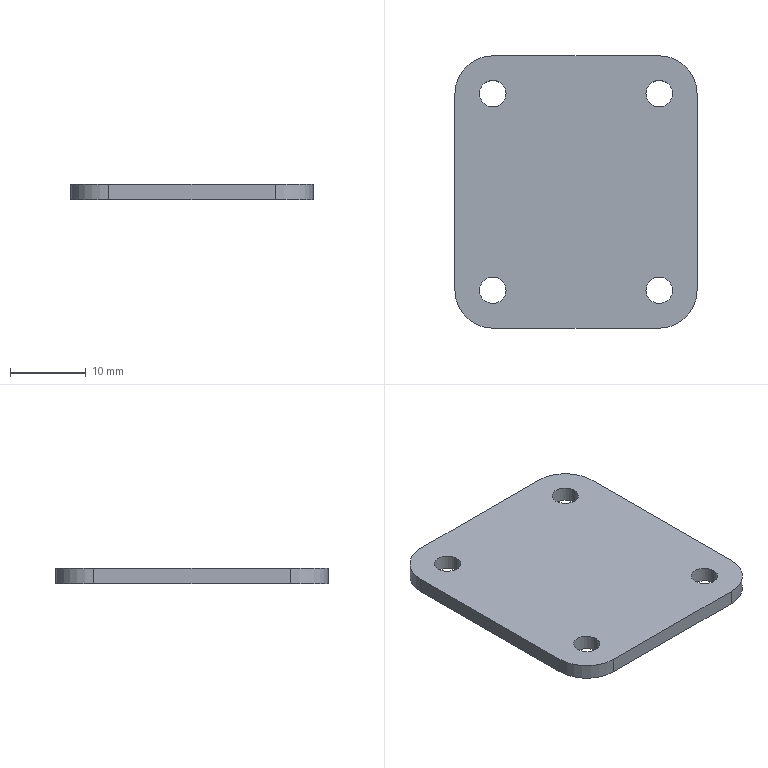Part | STEP file | YCD14007A-08.03.08.05 Engraving Plate | 1 solid | 18 faces | box 32 x 36 x 2 mm | volume 2184 mm3 | cylinder 12 | plane 6 | commonest cylinder face diameters 3.5 x8 10 x4
STEP:
#1=CARTESIAN_POINT('',(0.,0.,0.));
#2=DIRECTION('',(0.,0.,1.));
#3=DIRECTION('',(1.,0.,0.));
#4=AXIS2_PLACEMENT_3D('',#1,#2,#3);
#5=CARTESIAN_POINT('',(12.75,-13.,0.));
#6=VERTEX_POINT('',#5);
#7=CARTESIAN_POINT('',(12.75,-13.,2.));
#8=VERTEX_POINT('',#7);
#9=CARTESIAN_POINT('',(12.75,-13.,-0.001));
#10=DIRECTION('',(0.,0.,1.));
#11=VECTOR('',#10,1.);
#12=LINE('',#9,#11);
#13=CARTESIAN_POINT('',(11.,-13.,-0.001));
#14=DIRECTION('',(0.,0.,1.));
#15=DIRECTION('',(1.,0.,0.));
#16=AXIS2_PLACEMENT_3D('',#13,#14,#15);
#17=CYLINDRICAL_SURFACE('',#16,1.75);
#18=CARTESIAN_POINT('',(6.283,0.));
#19=DIRECTION('',(0.,1.));
#20=VECTOR('',#19,1.);
#21=LINE('',#18,#20);
#22=(GEOMETRIC_REPRESENTATION_CONTEXT(2)PARAMETRIC_REPRESENTATION_CONTEXT()REPRESENTATION_CONTEXT('',''));
#23=DEFINITIONAL_REPRESENTATION('',(#21),#22);
#24=PCURVE('',#17,#23);
#25=CARTESIAN_POINT('',(11.,-13.,-0.001));
#26=DIRECTION('',(0.,0.,1.));
#27=DIRECTION('',(1.,0.,0.));
#28=AXIS2_PLACEMENT_3D('',#25,#26,#27);
#29=CYLINDRICAL_SURFACE('',#28,1.75);
#30=CARTESIAN_POINT('',(0.,0.));
#31=DIRECTION('',(0.,1.));
#32=VECTOR('',#31,1.);
#33=LINE('',#30,#32);
#34=(GEOMETRIC_REPRESENTATION_CONTEXT(2)PARAMETRIC_REPRESENTATION_CONTEXT()REPRESENTATION_CONTEXT('',''));
#35=DEFINITIONAL_REPRESENTATION('',(#33),#34);
#36=PCURVE('',#29,#35);
#37=SURFACE_CURVE('',#12,(#24,#36),.PCURVE_S1.);
#38=EDGE_CURVE('',#6,#8,#37,.T.);
#39=ORIENTED_EDGE('',*,*,#38,.T.);
#40=CARTESIAN_POINT('',(9.25,-13.,2.));
#41=VERTEX_POINT('',#40);
#42=CARTESIAN_POINT('',(11.,-13.,2.));
#43=DIRECTION('',(0.,0.,1.));
#44=DIRECTION('',(1.,0.,0.));
#45=AXIS2_PLACEMENT_3D('',#42,#43,#44);
#46=CIRCLE('',#45,1.75);
#47=CARTESIAN_POINT('',(0.,2.001));
#48=DIRECTION('',(1.,0.));
#49=VECTOR('',#48,1.);
#50=LINE('',#47,#49);
#51=(GEOMETRIC_REPRESENTATION_CONTEXT(2)PARAMETRIC_REPRESENTATION_CONTEXT()REPRESENTATION_CONTEXT('',''));
#52=DEFINITIONAL_REPRESENTATION('',(#50),#51);
#53=PCURVE('',#17,#52);
#54=CARTESIAN_POINT('',(0.,0.,2.));
#55=DIRECTION('',(0.,0.,1.));
#56=DIRECTION('',(1.,0.,0.));
#57=AXIS2_PLACEMENT_3D('',#54,#55,#56);
#58=PLANE('',#57);
#59=CARTESIAN_POINT('',(11.,-13.));
#60=DIRECTION('',(1.,0.));
#61=AXIS2_PLACEMENT_2D('',#59,#60);
#62=CIRCLE('',#61,1.75);
#63=(GEOMETRIC_REPRESENTATION_CONTEXT(2)PARAMETRIC_REPRESENTATION_CONTEXT()REPRESENTATION_CONTEXT('',''));
#64=DEFINITIONAL_REPRESENTATION('',(#62),#63);
#65=PCURVE('',#58,#64);
#66=SURFACE_CURVE('',#46,(#53,#65),.PCURVE_S1.);
#67=EDGE_CURVE('',#41,#8,#66,.T.);
#68=ORIENTED_EDGE('',*,*,#67,.F.);
#69=CARTESIAN_POINT('',(9.25,-13.,0.));
#70=VERTEX_POINT('',#69);
#71=CARTESIAN_POINT('',(9.25,-13.,-0.001));
#72=DIRECTION('',(0.,0.,1.));
#73=VECTOR('',#72,1.);
#74=LINE('',#71,#73);
#75=CARTESIAN_POINT('',(3.142,0.));
#76=DIRECTION('',(0.,1.));
#77=VECTOR('',#76,1.);
#78=LINE('',#75,#77);
#79=(GEOMETRIC_REPRESENTATION_CONTEXT(2)PARAMETRIC_REPRESENTATION_CONTEXT()REPRESENTATION_CONTEXT('',''));
#80=DEFINITIONAL_REPRESENTATION('',(#78),#79);
#81=PCURVE('',#17,#80);
#82=CARTESIAN_POINT('',(3.142,0.));
#83=DIRECTION('',(0.,1.));
#84=VECTOR('',#83,1.);
#85=LINE('',#82,#84);
#86=(GEOMETRIC_REPRESENTATION_CONTEXT(2)PARAMETRIC_REPRESENTATION_CONTEXT()REPRESENTATION_CONTEXT('',''));
#87=DEFINITIONAL_REPRESENTATION('',(#85),#86);
#88=PCURVE('',#29,#87);
#89=SURFACE_CURVE('',#74,(#81,#88),.PCURVE_S1.);
#90=EDGE_CURVE('',#70,#41,#89,.T.);
#91=ORIENTED_EDGE('',*,*,#90,.F.);
#92=CARTESIAN_POINT('',(11.,-13.,0.));
#93=DIRECTION('',(0.,0.,-1.));
#94=DIRECTION('',(1.,0.,0.));
#95=AXIS2_PLACEMENT_3D('',#92,#93,#94);
#96=CIRCLE('',#95,1.75);
#97=CARTESIAN_POINT('',(6.283,0.001));
#98=DIRECTION('',(-1.,0.));
#99=VECTOR('',#98,1.);
#100=LINE('',#97,#99);
#101=(GEOMETRIC_REPRESENTATION_CONTEXT(2)PARAMETRIC_REPRESENTATION_CONTEXT()REPRESENTATION_CONTEXT('',''));
#102=DEFINITIONAL_REPRESENTATION('',(#100),#101);
#103=PCURVE('',#17,#102);
#104=CARTESIAN_POINT('',(0.,0.,0.));
#105=DIRECTION('',(0.,0.,1.));
#106=DIRECTION('',(1.,0.,0.));
#107=AXIS2_PLACEMENT_3D('',#104,#105,#106);
#108=PLANE('',#107);
#109=CARTESIAN_POINT('',(12.75,-13.));
#110=CARTESIAN_POINT('',(12.75,-16.031));
#111=CARTESIAN_POINT('',(10.125,-14.516));
#112=CARTESIAN_POINT('',(7.5,-13.));
#113=CARTESIAN_POINT('',(10.125,-11.484));
#114=CARTESIAN_POINT('',(12.75,-9.969));
#115=CARTESIAN_POINT('',(12.75,-13.));
#116=(BOUNDED_CURVE()B_SPLINE_CURVE(2,(#109,#110,#111,#112,#113,#114,#115),.UNSPECIFIED.,.T.,.F.)B_SPLINE_CURVE_WITH_KNOTS((1,2,2,2,2,1),(-2.094,0.,2.094,4.189,6.283,8.378),.UNSPECIFIED.)CURVE()GEOMETRIC_REPRESENTATION_ITEM()RATIONAL_B_SPLINE_CURVE((1.,0.5,1.,0.5,1.,0.5,1.))REPRESENTATION_ITEM(''));
#117=(GEOMETRIC_REPRESENTATION_CONTEXT(2)PARAMETRIC_REPRESENTATION_CONTEXT()REPRESENTATION_CONTEXT('',''));
#118=DEFINITIONAL_REPRESENTATION('',(#116),#117);
#119=PCURVE('',#108,#118);
#120=SURFACE_CURVE('',#96,(#103,#119),.PCURVE_S1.);
#121=EDGE_CURVE('',#6,#70,#120,.T.);
#122=ORIENTED_EDGE('',*,*,#121,.F.);
#123=EDGE_LOOP('',(#39,#68,#91,#122));
#124=FACE_BOUND('',#123,.F.);
#125=ADVANCED_FACE('',(#124),#17,.F.);
#126=CARTESIAN_POINT('',(-9.25,-13.,0.));
#127=VERTEX_POINT('',#126);
#128=CARTESIAN_POINT('',(-9.25,-13.,2.));
#129=VERTEX_POINT('',#128);
#130=CARTESIAN_POINT('',(-9.25,-13.,-0.001));
#131=DIRECTION('',(0.,0.,1.));
#132=VECTOR('',#131,1.);
#133=LINE('',#130,#132);
#134=CARTESIAN_POINT('',(-11.,-13.,-0.001));
#135=DIRECTION('',(0.,0.,1.));
#136=DIRECTION('',(1.,0.,0.));
#137=AXIS2_PLACEMENT_3D('',#134,#135,#136);
#138=CYLINDRICAL_SURFACE('',#137,1.75);
#139=CARTESIAN_POINT('',(6.283,0.));
#140=DIRECTION('',(0.,1.));
#141=VECTOR('',#140,1.);
#142=LINE('',#139,#141);
#143=(GEOMETRIC_REPRESENTATION_CONTEXT(2)PARAMETRIC_REPRESENTATION_CONTEXT()REPRESENTATION_CONTEXT('',''));
#144=DEFINITIONAL_REPRESENTATION('',(#142),#143);
#145=PCURVE('',#138,#144);
#146=CARTESIAN_POINT('',(-11.,-13.,-0.001));
#147=DIRECTION('',(0.,0.,1.));
#148=DIRECTION('',(1.,0.,0.));
#149=AXIS2_PLACEMENT_3D('',#146,#147,#148);
#150=CYLINDRICAL_SURFACE('',#149,1.75);
#151=CARTESIAN_POINT('',(0.,0.));
#152=DIRECTION('',(0.,1.));
#153=VECTOR('',#152,1.);
#154=LINE('',#151,#153);
#155=(GEOMETRIC_REPRESENTATION_CONTEXT(2)PARAMETRIC_REPRESENTATION_CONTEXT()REPRESENTATION_CONTEXT('',''));
#156=DEFINITIONAL_REPRESENTATION('',(#154),#155);
#157=PCURVE('',#150,#156);
#158=SURFACE_CURVE('',#133,(#145,#157),.PCURVE_S1.);
#159=EDGE_CURVE('',#127,#129,#158,.T.);
#160=ORIENTED_EDGE('',*,*,#159,.T.);
#161=CARTESIAN_POINT('',(-12.75,-13.,2.));
#162=VERTEX_POINT('',#161);
#163=CARTESIAN_POINT('',(-11.,-13.,2.));
#164=DIRECTION('',(0.,0.,1.));
#165=DIRECTION('',(1.,0.,0.));
#166=AXIS2_PLACEMENT_3D('',#163,#164,#165);
#167=CIRCLE('',#166,1.75);
#168=CARTESIAN_POINT('',(0.,2.001));
#169=DIRECTION('',(1.,0.));
#170=VECTOR('',#169,1.);
#171=LINE('',#168,#170);
#172=(GEOMETRIC_REPRESENTATION_CONTEXT(2)PARAMETRIC_REPRESENTATION_CONTEXT()REPRESENTATION_CONTEXT('',''));
#173=DEFINITIONAL_REPRESENTATION('',(#171),#172);
#174=PCURVE('',#138,#173);
#175=CARTESIAN_POINT('',(-11.,-13.));
#176=DIRECTION('',(1.,0.));
#177=AXIS2_PLACEMENT_2D('',#175,#176);
#178=CIRCLE('',#177,1.75);
#179=(GEOMETRIC_REPRESENTATION_CONTEXT(2)PARAMETRIC_REPRESENTATION_CONTEXT()REPRESENTATION_CONTEXT('',''));
#180=DEFINITIONAL_REPRESENTATION('',(#178),#179);
#181=PCURVE('',#58,#180);
#182=SURFACE_CURVE('',#167,(#174,#181),.PCURVE_S1.);
#183=EDGE_CURVE('',#162,#129,#182,.T.);
#184=ORIENTED_EDGE('',*,*,#183,.F.);
#185=CARTESIAN_POINT('',(-12.75,-13.,0.));
#186=VERTEX_POINT('',#185);
#187=CARTESIAN_POINT('',(-12.75,-13.,-0.001));
#188=DIRECTION('',(0.,0.,1.));
#189=VECTOR('',#188,1.);
#190=LINE('',#187,#189);
#191=CARTESIAN_POINT('',(3.142,0.));
#192=DIRECTION('',(0.,1.));
#193=VECTOR('',#192,1.);
#194=LINE('',#191,#193);
#195=(GEOMETRIC_REPRESENTATION_CONTEXT(2)PARAMETRIC_REPRESENTATION_CONTEXT()REPRESENTATION_CONTEXT('',''));
#196=DEFINITIONAL_REPRESENTATION('',(#194),#195);
#197=PCURVE('',#138,#196);
#198=CARTESIAN_POINT('',(3.142,0.));
#199=DIRECTION('',(0.,1.));
#200=VECTOR('',#199,1.);
#201=LINE('',#198,#200);
#202=(GEOMETRIC_REPRESENTATION_CONTEXT(2)PARAMETRIC_REPRESENTATION_CONTEXT()REPRESENTATION_CONTEXT('',''));
#203=DEFINITIONAL_REPRESENTATION('',(#201),#202);
#204=PCURVE('',#150,#203);
#205=SURFACE_CURVE('',#190,(#197,#204),.PCURVE_S1.);
#206=EDGE_CURVE('',#186,#162,#205,.T.);
#207=ORIENTED_EDGE('',*,*,#206,.F.);
#208=CARTESIAN_POINT('',(-11.,-13.,0.));
#209=DIRECTION('',(0.,0.,-1.));
#210=DIRECTION('',(1.,0.,0.));
#211=AXIS2_PLACEMENT_3D('',#208,#209,#210);
#212=CIRCLE('',#211,1.75);
#213=CARTESIAN_POINT('',(6.283,0.001));
#214=DIRECTION('',(-1.,0.));
#215=VECTOR('',#214,1.);
#216=LINE('',#213,#215);
#217=(GEOMETRIC_REPRESENTATION_CONTEXT(2)PARAMETRIC_REPRESENTATION_CONTEXT()REPRESENTATION_CONTEXT('',''));
#218=DEFINITIONAL_REPRESENTATION('',(#216),#217);
#219=PCURVE('',#138,#218);
#220=CARTESIAN_POINT('',(-9.25,-13.));
#221=CARTESIAN_POINT('',(-9.25,-16.031));
#222=CARTESIAN_POINT('',(-11.875,-14.516));
#223=CARTESIAN_POINT('',(-14.5,-13.));
#224=CARTESIAN_POINT('',(-11.875,-11.484));
#225=CARTESIAN_POINT('',(-9.25,-9.969));
#226=CARTESIAN_POINT('',(-9.25,-13.));
#227=(BOUNDED_CURVE()B_SPLINE_CURVE(2,(#220,#221,#222,#223,#224,#225,#226),.UNSPECIFIED.,.T.,.F.)B_SPLINE_CURVE_WITH_KNOTS((1,2,2,2,2,1),(-2.094,0.,2.094,4.189,6.283,8.378),.UNSPECIFIED.)CURVE()GEOMETRIC_REPRESENTATION_ITEM()RATIONAL_B_SPLINE_CURVE((1.,0.5,1.,0.5,1.,0.5,1.))REPRESENTATION_ITEM(''));
#228=(GEOMETRIC_REPRESENTATION_CONTEXT(2)PARAMETRIC_REPRESENTATION_CONTEXT()REPRESENTATION_CONTEXT('',''));
#229=DEFINITIONAL_REPRESENTATION('',(#227),#228);
#230=PCURVE('',#108,#229);
#231=SURFACE_CURVE('',#212,(#219,#230),.PCURVE_S1.);
#232=EDGE_CURVE('',#127,#186,#231,.T.);
#233=ORIENTED_EDGE('',*,*,#232,.F.);
#234=EDGE_LOOP('',(#160,#184,#207,#233));
#235=FACE_BOUND('',#234,.F.);
#236=ADVANCED_FACE('',(#235),#138,.F.);
#237=CARTESIAN_POINT('',(12.75,13.,0.));
#238=VERTEX_POINT('',#237);
#239=CARTESIAN_POINT('',(12.75,13.,2.));
#240=VERTEX_POINT('',#239);
#241=CARTESIAN_POINT('',(12.75,13.,-0.001));
#242=DIRECTION('',(0.,0.,1.));
#243=VECTOR('',#242,1.);
#244=LINE('',#241,#243);
#245=CARTESIAN_POINT('',(11.,13.,-0.001));
#246=DIRECTION('',(0.,0.,1.));
#247=DIRECTION('',(1.,0.,0.));
#248=AXIS2_PLACEMENT_3D('',#245,#246,#247);
#249=CYLINDRICAL_SURFACE('',#248,1.75);
#250=CARTESIAN_POINT('',(6.283,0.));
#251=DIRECTION('',(0.,1.));
#252=VECTOR('',#251,1.);
#253=LINE('',#250,#252);
#254=(GEOMETRIC_REPRESENTATION_CONTEXT(2)PARAMETRIC_REPRESENTATION_CONTEXT()REPRESENTATION_CONTEXT('',''));
#255=DEFINITIONAL_REPRESENTATION('',(#253),#254);
#256=PCURVE('',#249,#255);
#257=CARTESIAN_POINT('',(11.,13.,-0.001));
#258=DIRECTION('',(0.,0.,1.));
#259=DIRECTION('',(1.,0.,0.));
#260=AXIS2_PLACEMENT_3D('',#257,#258,#259);
#261=CYLINDRICAL_SURFACE('',#260,1.75);
#262=CARTESIAN_POINT('',(0.,0.));
#263=DIRECTION('',(0.,1.));
#264=VECTOR('',#263,1.);
#265=LINE('',#262,#264);
#266=(GEOMETRIC_REPRESENTATION_CONTEXT(2)PARAMETRIC_REPRESENTATION_CONTEXT()REPRESENTATION_CONTEXT('',''));
#267=DEFINITIONAL_REPRESENTATION('',(#265),#266);
#268=PCURVE('',#261,#267);
#269=SURFACE_CURVE('',#244,(#256,#268),.PCURVE_S1.);
#270=EDGE_CURVE('',#238,#240,#269,.T.);
#271=ORIENTED_EDGE('',*,*,#270,.T.);
#272=CARTESIAN_POINT('',(9.25,13.,2.));
#273=VERTEX_POINT('',#272);
#274=CARTESIAN_POINT('',(11.,13.,2.));
#275=DIRECTION('',(0.,0.,1.));
#276=DIRECTION('',(1.,0.,0.));
#277=AXIS2_PLACEMENT_3D('',#274,#275,#276);
#278=CIRCLE('',#277,1.75);
#279=CARTESIAN_POINT('',(0.,2.001));
#280=DIRECTION('',(1.,0.));
#281=VECTOR('',#280,1.);
#282=LINE('',#279,#281);
#283=(GEOMETRIC_REPRESENTATION_CONTEXT(2)PARAMETRIC_REPRESENTATION_CONTEXT()REPRESENTATION_CONTEXT('',''));
#284=DEFINITIONAL_REPRESENTATION('',(#282),#283);
#285=PCURVE('',#249,#284);
#286=CARTESIAN_POINT('',(11.,13.));
#287=DIRECTION('',(1.,0.));
#288=AXIS2_PLACEMENT_2D('',#286,#287);
#289=CIRCLE('',#288,1.75);
#290=(GEOMETRIC_REPRESENTATION_CONTEXT(2)PARAMETRIC_REPRESENTATION_CONTEXT()REPRESENTATION_CONTEXT('',''));
#291=DEFINITIONAL_REPRESENTATION('',(#289),#290);
#292=PCURVE('',#58,#291);
#293=SURFACE_CURVE('',#278,(#285,#292),.PCURVE_S1.);
#294=EDGE_CURVE('',#273,#240,#293,.T.);
#295=ORIENTED_EDGE('',*,*,#294,.F.);
#296=CARTESIAN_POINT('',(9.25,13.,0.));
#297=VERTEX_POINT('',#296);
#298=CARTESIAN_POINT('',(9.25,13.,-0.001));
#299=DIRECTION('',(0.,0.,1.));
#300=VECTOR('',#299,1.);
#301=LINE('',#298,#300);
#302=CARTESIAN_POINT('',(3.142,0.));
#303=DIRECTION('',(0.,1.));
#304=VECTOR('',#303,1.);
#305=LINE('',#302,#304);
#306=(GEOMETRIC_REPRESENTATION_CONTEXT(2)PARAMETRIC_REPRESENTATION_CONTEXT()REPRESENTATION_CONTEXT('',''));
#307=DEFINITIONAL_REPRESENTATION('',(#305),#306);
#308=PCURVE('',#249,#307);
#309=CARTESIAN_POINT('',(3.142,0.));
#310=DIRECTION('',(0.,1.));
#311=VECTOR('',#310,1.);
#312=LINE('',#309,#311);
#313=(GEOMETRIC_REPRESENTATION_CONTEXT(2)PARAMETRIC_REPRESENTATION_CONTEXT()REPRESENTATION_CONTEXT('',''));
#314=DEFINITIONAL_REPRESENTATION('',(#312),#313);
#315=PCURVE('',#261,#314);
#316=SURFACE_CURVE('',#301,(#308,#315),.PCURVE_S1.);
#317=EDGE_CURVE('',#297,#273,#316,.T.);
#318=ORIENTED_EDGE('',*,*,#317,.F.);
#319=CARTESIAN_POINT('',(11.,13.,0.));
#320=DIRECTION('',(0.,0.,-1.));
#321=DIRECTION('',(1.,0.,0.));
#322=AXIS2_PLACEMENT_3D('',#319,#320,#321);
#323=CIRCLE('',#322,1.75);
#324=CARTESIAN_POINT('',(6.283,0.001));
#325=DIRECTION('',(-1.,0.));
#326=VECTOR('',#325,1.);
#327=LINE('',#324,#326);
#328=(GEOMETRIC_REPRESENTATION_CONTEXT(2)PARAMETRIC_REPRESENTATION_CONTEXT()REPRESENTATION_CONTEXT('',''));
#329=DEFINITIONAL_REPRESENTATION('',(#327),#328);
#330=PCURVE('',#249,#329);
#331=CARTESIAN_POINT('',(12.75,13.));
#332=CARTESIAN_POINT('',(12.75,9.969));
#333=CARTESIAN_POINT('',(10.125,11.484));
#334=CARTESIAN_POINT('',(7.5,13.));
#335=CARTESIAN_POINT('',(10.125,14.516));
#336=CARTESIAN_POINT('',(12.75,16.031));
#337=CARTESIAN_POINT('',(12.75,13.));
#338=(BOUNDED_CURVE()B_SPLINE_CURVE(2,(#331,#332,#333,#334,#335,#336,#337),.UNSPECIFIED.,.T.,.F.)B_SPLINE_CURVE_WITH_KNOTS((1,2,2,2,2,1),(-2.094,0.,2.094,4.189,6.283,8.378),.UNSPECIFIED.)CURVE()GEOMETRIC_REPRESENTATION_ITEM()RATIONAL_B_SPLINE_CURVE((1.,0.5,1.,0.5,1.,0.5,1.))REPRESENTATION_ITEM(''));
#339=(GEOMETRIC_REPRESENTATION_CONTEXT(2)PARAMETRIC_REPRESENTATION_CONTEXT()REPRESENTATION_CONTEXT('',''));
#340=DEFINITIONAL_REPRESENTATION('',(#338),#339);
#341=PCURVE('',#108,#340);
#342=SURFACE_CURVE('',#323,(#330,#341),.PCURVE_S1.);
#343=EDGE_CURVE('',#238,#297,#342,.T.);
#344=ORIENTED_EDGE('',*,*,#343,.F.);
#345=EDGE_LOOP('',(#271,#295,#318,#344));
#346=FACE_BOUND('',#345,.F.);
#347=ADVANCED_FACE('',(#346),#249,.F.);
#348=CARTESIAN_POINT('',(-9.25,13.,0.));
#349=VERTEX_POINT('',#348);
#350=CARTESIAN_POINT('',(-9.25,13.,2.));
#351=VERTEX_POINT('',#350);
#352=CARTESIAN_POINT('',(-9.25,13.,-0.001));
#353=DIRECTION('',(0.,0.,1.));
#354=VECTOR('',#353,1.);
#355=LINE('',#352,#354);
#356=CARTESIAN_POINT('',(-11.,13.,-0.001));
#357=DIRECTION('',(0.,0.,1.));
#358=DIRECTION('',(1.,0.,0.));
#359=AXIS2_PLACEMENT_3D('',#356,#357,#358);
#360=CYLINDRICAL_SURFACE('',#359,1.75);
#361=CARTESIAN_POINT('',(6.283,0.));
#362=DIRECTION('',(0.,1.));
#363=VECTOR('',#362,1.);
#364=LINE('',#361,#363);
#365=(GEOMETRIC_REPRESENTATION_CONTEXT(2)PARAMETRIC_REPRESENTATION_CONTEXT()REPRESENTATION_CONTEXT('',''));
#366=DEFINITIONAL_REPRESENTATION('',(#364),#365);
#367=PCURVE('',#360,#366);
#368=CARTESIAN_POINT('',(-11.,13.,-0.001));
#369=DIRECTION('',(0.,0.,1.));
#370=DIRECTION('',(1.,0.,0.));
#371=AXIS2_PLACEMENT_3D('',#368,#369,#370);
#372=CYLINDRICAL_SURFACE('',#371,1.75);
#373=CARTESIAN_POINT('',(0.,0.));
#374=DIRECTION('',(0.,1.));
#375=VECTOR('',#374,1.);
#376=LINE('',#373,#375);
#377=(GEOMETRIC_REPRESENTATION_CONTEXT(2)PARAMETRIC_REPRESENTATION_CONTEXT()REPRESENTATION_CONTEXT('',''));
#378=DEFINITIONAL_REPRESENTATION('',(#376),#377);
#379=PCURVE('',#372,#378);
#380=SURFACE_CURVE('',#355,(#367,#379),.PCURVE_S1.);
#381=EDGE_CURVE('',#349,#351,#380,.T.);
#382=ORIENTED_EDGE('',*,*,#381,.T.);
#383=CARTESIAN_POINT('',(-12.75,13.,2.));
#384=VERTEX_POINT('',#383);
#385=CARTESIAN_POINT('',(-11.,13.,2.));
#386=DIRECTION('',(0.,0.,1.));
#387=DIRECTION('',(1.,0.,0.));
#388=AXIS2_PLACEMENT_3D('',#385,#386,#387);
#389=CIRCLE('',#388,1.75);
#390=CARTESIAN_POINT('',(0.,2.001));
#391=DIRECTION('',(1.,0.));
#392=VECTOR('',#391,1.);
#393=LINE('',#390,#392);
#394=(GEOMETRIC_REPRESENTATION_CONTEXT(2)PARAMETRIC_REPRESENTATION_CONTEXT()REPRESENTATION_CONTEXT('',''));
#395=DEFINITIONAL_REPRESENTATION('',(#393),#394);
#396=PCURVE('',#360,#395);
#397=CARTESIAN_POINT('',(-11.,13.));
#398=DIRECTION('',(1.,0.));
#399=AXIS2_PLACEMENT_2D('',#397,#398);
#400=CIRCLE('',#399,1.75);
#401=(GEOMETRIC_REPRESENTATION_CONTEXT(2)PARAMETRIC_REPRESENTATION_CONTEXT()REPRESENTATION_CONTEXT('',''));
#402=DEFINITIONAL_REPRESENTATION('',(#400),#401);
#403=PCURVE('',#58,#402);
#404=SURFACE_CURVE('',#389,(#396,#403),.PCURVE_S1.);
#405=EDGE_CURVE('',#384,#351,#404,.T.);
#406=ORIENTED_EDGE('',*,*,#405,.F.);
#407=CARTESIAN_POINT('',(-12.75,13.,0.));
#408=VERTEX_POINT('',#407);
#409=CARTESIAN_POINT('',(-12.75,13.,-0.001));
#410=DIRECTION('',(0.,0.,1.));
#411=VECTOR('',#410,1.);
#412=LINE('',#409,#411);
#413=CARTESIAN_POINT('',(3.142,0.));
#414=DIRECTION('',(0.,1.));
#415=VECTOR('',#414,1.);
#416=LINE('',#413,#415);
#417=(GEOMETRIC_REPRESENTATION_CONTEXT(2)PARAMETRIC_REPRESENTATION_CONTEXT()REPRESENTATION_CONTEXT('',''));
#418=DEFINITIONAL_REPRESENTATION('',(#416),#417);
#419=PCURVE('',#360,#418);
#420=CARTESIAN_POINT('',(3.142,0.));
#421=DIRECTION('',(0.,1.));
#422=VECTOR('',#421,1.);
#423=LINE('',#420,#422);
#424=(GEOMETRIC_REPRESENTATION_CONTEXT(2)PARAMETRIC_REPRESENTATION_CONTEXT()REPRESENTATION_CONTEXT('',''));
#425=DEFINITIONAL_REPRESENTATION('',(#423),#424);
#426=PCURVE('',#372,#425);
#427=SURFACE_CURVE('',#412,(#419,#426),.PCURVE_S1.);
#428=EDGE_CURVE('',#408,#384,#427,.T.);
#429=ORIENTED_EDGE('',*,*,#428,.F.);
#430=CARTESIAN_POINT('',(-11.,13.,0.));
#431=DIRECTION('',(0.,0.,-1.));
#432=DIRECTION('',(1.,0.,0.));
#433=AXIS2_PLACEMENT_3D('',#430,#431,#432);
#434=CIRCLE('',#433,1.75);
#435=CARTESIAN_POINT('',(6.283,0.001));
#436=DIRECTION('',(-1.,0.));
#437=VECTOR('',#436,1.);
#438=LINE('',#435,#437);
#439=(GEOMETRIC_REPRESENTATION_CONTEXT(2)PARAMETRIC_REPRESENTATION_CONTEXT()REPRESENTATION_CONTEXT('',''));
#440=DEFINITIONAL_REPRESENTATION('',(#438),#439);
#441=PCURVE('',#360,#440);
#442=CARTESIAN_POINT('',(-9.25,13.));
#443=CARTESIAN_POINT('',(-9.25,9.969));
#444=CARTESIAN_POINT('',(-11.875,11.484));
#445=CARTESIAN_POINT('',(-14.5,13.));
#446=CARTESIAN_POINT('',(-11.875,14.516));
#447=CARTESIAN_POINT('',(-9.25,16.031));
#448=CARTESIAN_POINT('',(-9.25,13.));
#449=(BOUNDED_CURVE()B_SPLINE_CURVE(2,(#442,#443,#444,#445,#446,#447,#448),.UNSPECIFIED.,.T.,.F.)B_SPLINE_CURVE_WITH_KNOTS((1,2,2,2,2,1),(-2.094,0.,2.094,4.189,6.283,8.378),.UNSPECIFIED.)CURVE()GEOMETRIC_REPRESENTATION_ITEM()RATIONAL_B_SPLINE_CURVE((1.,0.5,1.,0.5,1.,0.5,1.))REPRESENTATION_ITEM(''));
#450=(GEOMETRIC_REPRESENTATION_CONTEXT(2)PARAMETRIC_REPRESENTATION_CONTEXT()REPRESENTATION_CONTEXT('',''));
#451=DEFINITIONAL_REPRESENTATION('',(#449),#450);
#452=PCURVE('',#108,#451);
#453=SURFACE_CURVE('',#434,(#441,#452),.PCURVE_S1.);
#454=EDGE_CURVE('',#349,#408,#453,.T.);
#455=ORIENTED_EDGE('',*,*,#454,.F.);
#456=EDGE_LOOP('',(#382,#406,#429,#455));
#457=FACE_BOUND('',#456,.F.);
#458=ADVANCED_FACE('',(#457),#360,.F.);
#459=CARTESIAN_POINT('',(16.,-13.,2.));
#460=VERTEX_POINT('',#459);
#461=CARTESIAN_POINT('',(16.,13.,2.));
#462=VERTEX_POINT('',#461);
#463=CARTESIAN_POINT('',(16.,18.,2.));
#464=DIRECTION('',(0.,1.,0.));
#465=VECTOR('',#464,1.);
#466=LINE('',#463,#465);
#467=CARTESIAN_POINT('',(16.,18.,2.));
#468=DIRECTION('',(-1.,0.,0.));
#469=DIRECTION('',(0.,-1.,0.));
#470=AXIS2_PLACEMENT_3D('',#467,#468,#469);
#471=PLANE('',#470);
#472=CARTESIAN_POINT('',(0.,0.));
#473=DIRECTION('',(-1.,0.));
#474=VECTOR('',#473,1.);
#475=LINE('',#472,#474);
#476=(GEOMETRIC_REPRESENTATION_CONTEXT(2)PARAMETRIC_REPRESENTATION_CONTEXT()REPRESENTATION_CONTEXT('',''));
#477=DEFINITIONAL_REPRESENTATION('',(#475),#476);
#478=PCURVE('',#471,#477);
#479=CARTESIAN_POINT('',(16.,18.));
#480=DIRECTION('',(0.,1.));
#481=VECTOR('',#480,1.);
#482=LINE('',#479,#481);
#483=(GEOMETRIC_REPRESENTATION_CONTEXT(2)PARAMETRIC_REPRESENTATION_CONTEXT()REPRESENTATION_CONTEXT('',''));
#484=DEFINITIONAL_REPRESENTATION('',(#482),#483);
#485=PCURVE('',#58,#484);
#486=SURFACE_CURVE('',#466,(#478,#485),.PCURVE_S1.);
#487=EDGE_CURVE('',#460,#462,#486,.T.);
#488=ORIENTED_EDGE('',*,*,#487,.F.);
#489=CARTESIAN_POINT('',(16.,-13.,0.));
#490=VERTEX_POINT('',#489);
#491=CARTESIAN_POINT('',(16.,-13.,2.));
#492=DIRECTION('',(0.,0.,-1.));
#493=VECTOR('',#492,1.);
#494=LINE('',#491,#493);
#495=CARTESIAN_POINT('',(31.,0.));
#496=DIRECTION('',(0.,-1.));
#497=VECTOR('',#496,1.);
#498=LINE('',#495,#497);
#499=(GEOMETRIC_REPRESENTATION_CONTEXT(2)PARAMETRIC_REPRESENTATION_CONTEXT()REPRESENTATION_CONTEXT('',''));
#500=DEFINITIONAL_REPRESENTATION('',(#498),#499);
#501=PCURVE('',#471,#500);
#502=CARTESIAN_POINT('',(11.,-13.,2.));
#503=DIRECTION('',(0.,0.,-1.));
#504=DIRECTION('',(-1.,0.,0.));
#505=AXIS2_PLACEMENT_3D('',#502,#503,#504);
#506=CYLINDRICAL_SURFACE('',#505,5.);
#507=CARTESIAN_POINT('',(3.142,0.));
#508=DIRECTION('',(0.,1.));
#509=VECTOR('',#508,1.);
#510=LINE('',#507,#509);
#511=(GEOMETRIC_REPRESENTATION_CONTEXT(2)PARAMETRIC_REPRESENTATION_CONTEXT()REPRESENTATION_CONTEXT('',''));
#512=DEFINITIONAL_REPRESENTATION('',(#510),#511);
#513=PCURVE('',#506,#512);
#514=SURFACE_CURVE('',#494,(#501,#513),.PCURVE_S1.);
#515=EDGE_CURVE('',#460,#490,#514,.T.);
#516=ORIENTED_EDGE('',*,*,#515,.T.);
#517=CARTESIAN_POINT('',(16.,13.,0.));
#518=VERTEX_POINT('',#517);
#519=CARTESIAN_POINT('',(16.,18.,0.));
#520=DIRECTION('',(0.,1.,0.));
#521=VECTOR('',#520,1.);
#522=LINE('',#519,#521);
#523=CARTESIAN_POINT('',(0.,-2.));
#524=DIRECTION('',(-1.,0.));
#525=VECTOR('',#524,1.);
#526=LINE('',#523,#525);
#527=(GEOMETRIC_REPRESENTATION_CONTEXT(2)PARAMETRIC_REPRESENTATION_CONTEXT()REPRESENTATION_CONTEXT('',''));
#528=DEFINITIONAL_REPRESENTATION('',(#526),#527);
#529=PCURVE('',#471,#528);
#530=CARTESIAN_POINT('',(16.,18.));
#531=DIRECTION('',(0.,1.));
#532=VECTOR('',#531,1.);
#533=LINE('',#530,#532);
#534=(GEOMETRIC_REPRESENTATION_CONTEXT(2)PARAMETRIC_REPRESENTATION_CONTEXT()REPRESENTATION_CONTEXT('',''));
#535=DEFINITIONAL_REPRESENTATION('',(#533),#534);
#536=PCURVE('',#108,#535);
#537=SURFACE_CURVE('',#522,(#529,#536),.PCURVE_S1.);
#538=EDGE_CURVE('',#490,#518,#537,.T.);
#539=ORIENTED_EDGE('',*,*,#538,.T.);
#540=CARTESIAN_POINT('',(16.,13.,2.));
#541=DIRECTION('',(0.,0.,1.));
#542=VECTOR('',#541,1.);
#543=LINE('',#540,#542);
#544=CARTESIAN_POINT('',(5.,0.));
#545=DIRECTION('',(0.,1.));
#546=VECTOR('',#545,1.);
#547=LINE('',#544,#546);
#548=(GEOMETRIC_REPRESENTATION_CONTEXT(2)PARAMETRIC_REPRESENTATION_CONTEXT()REPRESENTATION_CONTEXT('',''));
#549=DEFINITIONAL_REPRESENTATION('',(#547),#548);
#550=PCURVE('',#471,#549);
#551=CARTESIAN_POINT('',(11.,13.,2.));
#552=DIRECTION('',(0.,0.,-1.));
#553=DIRECTION('',(-1.,0.,0.));
#554=AXIS2_PLACEMENT_3D('',#551,#552,#553);
#555=CYLINDRICAL_SURFACE('',#554,5.);
#556=CARTESIAN_POINT('',(3.142,0.));
#557=DIRECTION('',(0.,-1.));
#558=VECTOR('',#557,1.);
#559=LINE('',#556,#558);
#560=(GEOMETRIC_REPRESENTATION_CONTEXT(2)PARAMETRIC_REPRESENTATION_CONTEXT()REPRESENTATION_CONTEXT('',''));
#561=DEFINITIONAL_REPRESENTATION('',(#559),#560);
#562=PCURVE('',#555,#561);
#563=SURFACE_CURVE('',#543,(#550,#562),.PCURVE_S1.);
#564=EDGE_CURVE('',#518,#462,#563,.T.);
#565=ORIENTED_EDGE('',*,*,#564,.T.);
#566=EDGE_LOOP('',(#488,#516,#539,#565));
#567=FACE_BOUND('',#566,.T.);
#568=ADVANCED_FACE('',(#567),#471,.F.);
#569=CARTESIAN_POINT('',(11.,18.,2.));
#570=VERTEX_POINT('',#569);
#571=CARTESIAN_POINT('',(-11.,18.,2.));
#572=VERTEX_POINT('',#571);
#573=CARTESIAN_POINT('',(-16.,18.,2.));
#574=DIRECTION('',(-1.,0.,0.));
#575=VECTOR('',#574,1.);
#576=LINE('',#573,#575);
#577=CARTESIAN_POINT('',(-16.,18.,2.));
#578=DIRECTION('',(0.,-1.,0.));
#579=DIRECTION('',(0.,0.,-1.));
#580=AXIS2_PLACEMENT_3D('',#577,#578,#579);
#581=PLANE('',#580);
#582=CARTESIAN_POINT('',(0.,0.));
#583=DIRECTION('',(0.,-1.));
#584=VECTOR('',#583,1.);
#585=LINE('',#582,#584);
#586=(GEOMETRIC_REPRESENTATION_CONTEXT(2)PARAMETRIC_REPRESENTATION_CONTEXT()REPRESENTATION_CONTEXT('',''));
#587=DEFINITIONAL_REPRESENTATION('',(#585),#586);
#588=PCURVE('',#581,#587);
#589=CARTESIAN_POINT('',(-16.,18.));
#590=DIRECTION('',(-1.,0.));
#591=VECTOR('',#590,1.);
#592=LINE('',#589,#591);
#593=(GEOMETRIC_REPRESENTATION_CONTEXT(2)PARAMETRIC_REPRESENTATION_CONTEXT()REPRESENTATION_CONTEXT('',''));
#594=DEFINITIONAL_REPRESENTATION('',(#592),#593);
#595=PCURVE('',#58,#594);
#596=SURFACE_CURVE('',#576,(#588,#595),.PCURVE_S1.);
#597=EDGE_CURVE('',#570,#572,#596,.T.);
#598=ORIENTED_EDGE('',*,*,#597,.F.);
#599=CARTESIAN_POINT('',(11.,18.,0.));
#600=VERTEX_POINT('',#599);
#601=CARTESIAN_POINT('',(11.,18.,2.));
#602=DIRECTION('',(0.,0.,-1.));
#603=VECTOR('',#602,1.);
#604=LINE('',#601,#603);
#605=CARTESIAN_POINT('',(0.,27.));
#606=DIRECTION('',(1.,0.));
#607=VECTOR('',#606,1.);
#608=LINE('',#605,#607);
#609=(GEOMETRIC_REPRESENTATION_CONTEXT(2)PARAMETRIC_REPRESENTATION_CONTEXT()REPRESENTATION_CONTEXT('',''));
#610=DEFINITIONAL_REPRESENTATION('',(#608),#609);
#611=PCURVE('',#581,#610);
#612=CARTESIAN_POINT('',(1.571,0.));
#613=DIRECTION('',(0.,1.));
#614=VECTOR('',#613,1.);
#615=LINE('',#612,#614);
#616=(GEOMETRIC_REPRESENTATION_CONTEXT(2)PARAMETRIC_REPRESENTATION_CONTEXT()REPRESENTATION_CONTEXT('',''));
#617=DEFINITIONAL_REPRESENTATION('',(#615),#616);
#618=PCURVE('',#555,#617);
#619=SURFACE_CURVE('',#604,(#611,#618),.PCURVE_S1.);
#620=EDGE_CURVE('',#570,#600,#619,.T.);
#621=ORIENTED_EDGE('',*,*,#620,.T.);
#622=CARTESIAN_POINT('',(-11.,18.,0.));
#623=VERTEX_POINT('',#622);
#624=CARTESIAN_POINT('',(-16.,18.,0.));
#625=DIRECTION('',(-1.,0.,0.));
#626=VECTOR('',#625,1.);
#627=LINE('',#624,#626);
#628=CARTESIAN_POINT('',(2.,0.));
#629=DIRECTION('',(0.,-1.));
#630=VECTOR('',#629,1.);
#631=LINE('',#628,#630);
#632=(GEOMETRIC_REPRESENTATION_CONTEXT(2)PARAMETRIC_REPRESENTATION_CONTEXT()REPRESENTATION_CONTEXT('',''));
#633=DEFINITIONAL_REPRESENTATION('',(#631),#632);
#634=PCURVE('',#581,#633);
#635=CARTESIAN_POINT('',(-16.,18.));
#636=DIRECTION('',(-1.,0.));
#637=VECTOR('',#636,1.);
#638=LINE('',#635,#637);
#639=(GEOMETRIC_REPRESENTATION_CONTEXT(2)PARAMETRIC_REPRESENTATION_CONTEXT()REPRESENTATION_CONTEXT('',''));
#640=DEFINITIONAL_REPRESENTATION('',(#638),#639);
#641=PCURVE('',#108,#640);
#642=SURFACE_CURVE('',#627,(#634,#641),.PCURVE_S1.);
#643=EDGE_CURVE('',#600,#623,#642,.T.);
#644=ORIENTED_EDGE('',*,*,#643,.T.);
#645=CARTESIAN_POINT('',(-11.,18.,2.));
#646=DIRECTION('',(0.,0.,1.));
#647=VECTOR('',#646,1.);
#648=LINE('',#645,#647);
#649=CARTESIAN_POINT('',(0.,5.));
#650=DIRECTION('',(-1.,0.));
#651=VECTOR('',#650,1.);
#652=LINE('',#649,#651);
#653=(GEOMETRIC_REPRESENTATION_CONTEXT(2)PARAMETRIC_REPRESENTATION_CONTEXT()REPRESENTATION_CONTEXT('',''));
#654=DEFINITIONAL_REPRESENTATION('',(#652),#653);
#655=PCURVE('',#581,#654);
#656=CARTESIAN_POINT('',(-11.,13.,2.));
#657=DIRECTION('',(0.,0.,-1.));
#658=DIRECTION('',(-1.,0.,0.));
#659=AXIS2_PLACEMENT_3D('',#656,#657,#658);
#660=CYLINDRICAL_SURFACE('',#659,5.);
#661=CARTESIAN_POINT('',(1.571,0.));
#662=DIRECTION('',(0.,-1.));
#663=VECTOR('',#662,1.);
#664=LINE('',#661,#663);
#665=(GEOMETRIC_REPRESENTATION_CONTEXT(2)PARAMETRIC_REPRESENTATION_CONTEXT()REPRESENTATION_CONTEXT('',''));
#666=DEFINITIONAL_REPRESENTATION('',(#664),#665);
#667=PCURVE('',#660,#666);
#668=SURFACE_CURVE('',#648,(#655,#667),.PCURVE_S1.);
#669=EDGE_CURVE('',#623,#572,#668,.T.);
#670=ORIENTED_EDGE('',*,*,#669,.T.);
#671=EDGE_LOOP('',(#598,#621,#644,#670));
#672=FACE_BOUND('',#671,.T.);
#673=ADVANCED_FACE('',(#672),#581,.F.);
#674=CARTESIAN_POINT('',(-16.,13.,0.));
#675=VERTEX_POINT('',#674);
#676=CARTESIAN_POINT('',(-16.,-13.,0.));
#677=VERTEX_POINT('',#676);
#678=CARTESIAN_POINT('',(-16.,18.,0.));
#679=DIRECTION('',(0.,-1.,0.));
#680=VECTOR('',#679,1.);
#681=LINE('',#678,#680);
#682=CARTESIAN_POINT('',(-16.,18.,2.));
#683=DIRECTION('',(1.,0.,0.));
#684=DIRECTION('',(0.,1.,0.));
#685=AXIS2_PLACEMENT_3D('',#682,#683,#684);
#686=PLANE('',#685);
#687=CARTESIAN_POINT('',(0.,-2.));
#688=DIRECTION('',(-1.,0.));
#689=VECTOR('',#688,1.);
#690=LINE('',#687,#689);
#691=(GEOMETRIC_REPRESENTATION_CONTEXT(2)PARAMETRIC_REPRESENTATION_CONTEXT()REPRESENTATION_CONTEXT('',''));
#692=DEFINITIONAL_REPRESENTATION('',(#690),#691);
#693=PCURVE('',#686,#692);
#694=CARTESIAN_POINT('',(-16.,18.));
#695=DIRECTION('',(0.,-1.));
#696=VECTOR('',#695,1.);
#697=LINE('',#694,#696);
#698=(GEOMETRIC_REPRESENTATION_CONTEXT(2)PARAMETRIC_REPRESENTATION_CONTEXT()REPRESENTATION_CONTEXT('',''));
#699=DEFINITIONAL_REPRESENTATION('',(#697),#698);
#700=PCURVE('',#108,#699);
#701=SURFACE_CURVE('',#681,(#693,#700),.PCURVE_S1.);
#702=EDGE_CURVE('',#675,#677,#701,.T.);
#703=ORIENTED_EDGE('',*,*,#702,.T.);
#704=CARTESIAN_POINT('',(-16.,-13.,2.));
#705=VERTEX_POINT('',#704);
#706=CARTESIAN_POINT('',(-16.,-13.,2.));
#707=DIRECTION('',(0.,0.,1.));
#708=VECTOR('',#707,1.);
#709=LINE('',#706,#708);
#710=CARTESIAN_POINT('',(-31.,0.));
#711=DIRECTION('',(0.,1.));
#712=VECTOR('',#711,1.);
#713=LINE('',#710,#712);
#714=(GEOMETRIC_REPRESENTATION_CONTEXT(2)PARAMETRIC_REPRESENTATION_CONTEXT()REPRESENTATION_CONTEXT('',''));
#715=DEFINITIONAL_REPRESENTATION('',(#713),#714);
#716=PCURVE('',#686,#715);
#717=CARTESIAN_POINT('',(-11.,-13.,2.));
#718=DIRECTION('',(0.,0.,-1.));
#719=DIRECTION('',(-1.,0.,0.));
#720=AXIS2_PLACEMENT_3D('',#717,#718,#719);
#721=CYLINDRICAL_SURFACE('',#720,5.);
#722=CARTESIAN_POINT('',(6.283,0.));
#723=DIRECTION('',(0.,-1.));
#724=VECTOR('',#723,1.);
#725=LINE('',#722,#724);
#726=(GEOMETRIC_REPRESENTATION_CONTEXT(2)PARAMETRIC_REPRESENTATION_CONTEXT()REPRESENTATION_CONTEXT('',''));
#727=DEFINITIONAL_REPRESENTATION('',(#725),#726);
#728=PCURVE('',#721,#727);
#729=SURFACE_CURVE('',#709,(#716,#728),.PCURVE_S1.);
#730=EDGE_CURVE('',#677,#705,#729,.T.);
#731=ORIENTED_EDGE('',*,*,#730,.T.);
#732=CARTESIAN_POINT('',(-16.,13.,2.));
#733=VERTEX_POINT('',#732);
#734=CARTESIAN_POINT('',(-16.,18.,2.));
#735=DIRECTION('',(0.,-1.,0.));
#736=VECTOR('',#735,1.);
#737=LINE('',#734,#736);
#738=CARTESIAN_POINT('',(0.,0.));
#739=DIRECTION('',(-1.,0.));
#740=VECTOR('',#739,1.);
#741=LINE('',#738,#740);
#742=(GEOMETRIC_REPRESENTATION_CONTEXT(2)PARAMETRIC_REPRESENTATION_CONTEXT()REPRESENTATION_CONTEXT('',''));
#743=DEFINITIONAL_REPRESENTATION('',(#741),#742);
#744=PCURVE('',#686,#743);
#745=CARTESIAN_POINT('',(-16.,18.));
#746=DIRECTION('',(0.,-1.));
#747=VECTOR('',#746,1.);
#748=LINE('',#745,#747);
#749=(GEOMETRIC_REPRESENTATION_CONTEXT(2)PARAMETRIC_REPRESENTATION_CONTEXT()REPRESENTATION_CONTEXT('',''));
#750=DEFINITIONAL_REPRESENTATION('',(#748),#749);
#751=PCURVE('',#58,#750);
#752=SURFACE_CURVE('',#737,(#744,#751),.PCURVE_S1.);
#753=EDGE_CURVE('',#733,#705,#752,.T.);
#754=ORIENTED_EDGE('',*,*,#753,.F.);
#755=CARTESIAN_POINT('',(-16.,13.,2.));
#756=DIRECTION('',(0.,0.,-1.));
#757=VECTOR('',#756,1.);
#758=LINE('',#755,#757);
#759=CARTESIAN_POINT('',(-5.,0.));
#760=DIRECTION('',(0.,-1.));
#761=VECTOR('',#760,1.);
#762=LINE('',#759,#761);
#763=(GEOMETRIC_REPRESENTATION_CONTEXT(2)PARAMETRIC_REPRESENTATION_CONTEXT()REPRESENTATION_CONTEXT('',''));
#764=DEFINITIONAL_REPRESENTATION('',(#762),#763);
#765=PCURVE('',#686,#764);
#766=CARTESIAN_POINT('',(0.,0.));
#767=DIRECTION('',(0.,1.));
#768=VECTOR('',#767,1.);
#769=LINE('',#766,#768);
#770=(GEOMETRIC_REPRESENTATION_CONTEXT(2)PARAMETRIC_REPRESENTATION_CONTEXT()REPRESENTATION_CONTEXT('',''));
#771=DEFINITIONAL_REPRESENTATION('',(#769),#770);
#772=PCURVE('',#660,#771);
#773=SURFACE_CURVE('',#758,(#765,#772),.PCURVE_S1.);
#774=EDGE_CURVE('',#733,#675,#773,.T.);
#775=ORIENTED_EDGE('',*,*,#774,.T.);
#776=EDGE_LOOP('',(#703,#731,#754,#775));
#777=FACE_BOUND('',#776,.T.);
#778=ADVANCED_FACE('',(#777),#686,.F.);
#779=CARTESIAN_POINT('',(-11.,-18.,0.));
#780=VERTEX_POINT('',#779);
#781=CARTESIAN_POINT('',(11.,-18.,0.));
#782=VERTEX_POINT('',#781);
#783=CARTESIAN_POINT('',(-16.,-18.,0.));
#784=DIRECTION('',(1.,0.,0.));
#785=VECTOR('',#784,1.);
#786=LINE('',#783,#785);
#787=CARTESIAN_POINT('',(-16.,-18.,2.));
#788=DIRECTION('',(0.,1.,0.));
#789=DIRECTION('',(0.,0.,1.));
#790=AXIS2_PLACEMENT_3D('',#787,#788,#789);
#791=PLANE('',#790);
#792=CARTESIAN_POINT('',(-2.,0.));
#793=DIRECTION('',(0.,1.));
#794=VECTOR('',#793,1.);
#795=LINE('',#792,#794);
#796=(GEOMETRIC_REPRESENTATION_CONTEXT(2)PARAMETRIC_REPRESENTATION_CONTEXT()REPRESENTATION_CONTEXT('',''));
#797=DEFINITIONAL_REPRESENTATION('',(#795),#796);
#798=PCURVE('',#791,#797);
#799=CARTESIAN_POINT('',(-16.,-18.));
#800=DIRECTION('',(1.,0.));
#801=VECTOR('',#800,1.);
#802=LINE('',#799,#801);
#803=(GEOMETRIC_REPRESENTATION_CONTEXT(2)PARAMETRIC_REPRESENTATION_CONTEXT()REPRESENTATION_CONTEXT('',''));
#804=DEFINITIONAL_REPRESENTATION('',(#802),#803);
#805=PCURVE('',#108,#804);
#806=SURFACE_CURVE('',#786,(#798,#805),.PCURVE_S1.);
#807=EDGE_CURVE('',#780,#782,#806,.T.);
#808=ORIENTED_EDGE('',*,*,#807,.T.);
#809=CARTESIAN_POINT('',(11.,-18.,2.));
#810=VERTEX_POINT('',#809);
#811=CARTESIAN_POINT('',(11.,-18.,2.));
#812=DIRECTION('',(0.,0.,1.));
#813=VECTOR('',#812,1.);
#814=LINE('',#811,#813);
#815=CARTESIAN_POINT('',(0.,27.));
#816=DIRECTION('',(1.,0.));
#817=VECTOR('',#816,1.);
#818=LINE('',#815,#817);
#819=(GEOMETRIC_REPRESENTATION_CONTEXT(2)PARAMETRIC_REPRESENTATION_CONTEXT()REPRESENTATION_CONTEXT('',''));
#820=DEFINITIONAL_REPRESENTATION('',(#818),#819);
#821=PCURVE('',#791,#820);
#822=CARTESIAN_POINT('',(4.712,0.));
#823=DIRECTION('',(0.,-1.));
#824=VECTOR('',#823,1.);
#825=LINE('',#822,#824);
#826=(GEOMETRIC_REPRESENTATION_CONTEXT(2)PARAMETRIC_REPRESENTATION_CONTEXT()REPRESENTATION_CONTEXT('',''));
#827=DEFINITIONAL_REPRESENTATION('',(#825),#826);
#828=PCURVE('',#506,#827);
#829=SURFACE_CURVE('',#814,(#821,#828),.PCURVE_S1.);
#830=EDGE_CURVE('',#782,#810,#829,.T.);
#831=ORIENTED_EDGE('',*,*,#830,.T.);
#832=CARTESIAN_POINT('',(-11.,-18.,2.));
#833=VERTEX_POINT('',#832);
#834=CARTESIAN_POINT('',(-16.,-18.,2.));
#835=DIRECTION('',(1.,0.,0.));
#836=VECTOR('',#835,1.);
#837=LINE('',#834,#836);
#838=CARTESIAN_POINT('',(0.,0.));
#839=DIRECTION('',(0.,1.));
#840=VECTOR('',#839,1.);
#841=LINE('',#838,#840);
#842=(GEOMETRIC_REPRESENTATION_CONTEXT(2)PARAMETRIC_REPRESENTATION_CONTEXT()REPRESENTATION_CONTEXT('',''));
#843=DEFINITIONAL_REPRESENTATION('',(#841),#842);
#844=PCURVE('',#791,#843);
#845=CARTESIAN_POINT('',(-16.,-18.));
#846=DIRECTION('',(1.,0.));
#847=VECTOR('',#846,1.);
#848=LINE('',#845,#847);
#849=(GEOMETRIC_REPRESENTATION_CONTEXT(2)PARAMETRIC_REPRESENTATION_CONTEXT()REPRESENTATION_CONTEXT('',''));
#850=DEFINITIONAL_REPRESENTATION('',(#848),#849);
#851=PCURVE('',#58,#850);
#852=SURFACE_CURVE('',#837,(#844,#851),.PCURVE_S1.);
#853=EDGE_CURVE('',#833,#810,#852,.T.);
#854=ORIENTED_EDGE('',*,*,#853,.F.);
#855=CARTESIAN_POINT('',(-11.,-18.,2.));
#856=DIRECTION('',(0.,0.,-1.));
#857=VECTOR('',#856,1.);
#858=LINE('',#855,#857);
#859=CARTESIAN_POINT('',(0.,5.));
#860=DIRECTION('',(-1.,0.));
#861=VECTOR('',#860,1.);
#862=LINE('',#859,#861);
#863=(GEOMETRIC_REPRESENTATION_CONTEXT(2)PARAMETRIC_REPRESENTATION_CONTEXT()REPRESENTATION_CONTEXT('',''));
#864=DEFINITIONAL_REPRESENTATION('',(#862),#863);
#865=PCURVE('',#791,#864);
#866=CARTESIAN_POINT('',(4.712,0.));
#867=DIRECTION('',(0.,1.));
#868=VECTOR('',#867,1.);
#869=LINE('',#866,#868);
#870=(GEOMETRIC_REPRESENTATION_CONTEXT(2)PARAMETRIC_REPRESENTATION_CONTEXT()REPRESENTATION_CONTEXT('',''));
#871=DEFINITIONAL_REPRESENTATION('',(#869),#870);
#872=PCURVE('',#721,#871);
#873=SURFACE_CURVE('',#858,(#865,#872),.PCURVE_S1.);
#874=EDGE_CURVE('',#833,#780,#873,.T.);
#875=ORIENTED_EDGE('',*,*,#874,.T.);
#876=EDGE_LOOP('',(#808,#831,#854,#875));
#877=FACE_BOUND('',#876,.T.);
#878=ADVANCED_FACE('',(#877),#791,.F.);
#879=CARTESIAN_POINT('',(11.,-13.,2.));
#880=DIRECTION('',(0.,0.,1.));
#881=DIRECTION('',(1.,0.,0.));
#882=AXIS2_PLACEMENT_3D('',#879,#880,#881);
#883=CIRCLE('',#882,1.75);
#884=CARTESIAN_POINT('',(11.,-13.));
#885=DIRECTION('',(1.,0.));
#886=AXIS2_PLACEMENT_2D('',#884,#885);
#887=CIRCLE('',#886,1.75);
#888=(GEOMETRIC_REPRESENTATION_CONTEXT(2)PARAMETRIC_REPRESENTATION_CONTEXT()REPRESENTATION_CONTEXT('',''));
#889=DEFINITIONAL_REPRESENTATION('',(#887),#888);
#890=PCURVE('',#58,#889);
#891=CARTESIAN_POINT('',(0.,2.001));
#892=DIRECTION('',(1.,0.));
#893=VECTOR('',#892,1.);
#894=LINE('',#891,#893);
#895=(GEOMETRIC_REPRESENTATION_CONTEXT(2)PARAMETRIC_REPRESENTATION_CONTEXT()REPRESENTATION_CONTEXT('',''));
#896=DEFINITIONAL_REPRESENTATION('',(#894),#895);
#897=PCURVE('',#29,#896);
#898=SURFACE_CURVE('',#883,(#890,#897),.PCURVE_S1.);
#899=EDGE_CURVE('',#8,#41,#898,.T.);
#900=ORIENTED_EDGE('',*,*,#899,.F.);
#901=ORIENTED_EDGE('',*,*,#67,.F.);
#902=EDGE_LOOP('',(#900,#901));
#903=FACE_BOUND('',#902,.T.);
#904=CARTESIAN_POINT('',(-11.,-13.,2.));
#905=DIRECTION('',(0.,0.,1.));
#906=DIRECTION('',(1.,0.,0.));
#907=AXIS2_PLACEMENT_3D('',#904,#905,#906);
#908=CIRCLE('',#907,1.75);
#909=CARTESIAN_POINT('',(-11.,-13.));
#910=DIRECTION('',(1.,0.));
#911=AXIS2_PLACEMENT_2D('',#909,#910);
#912=CIRCLE('',#911,1.75);
#913=(GEOMETRIC_REPRESENTATION_CONTEXT(2)PARAMETRIC_REPRESENTATION_CONTEXT()REPRESENTATION_CONTEXT('',''));
#914=DEFINITIONAL_REPRESENTATION('',(#912),#913);
#915=PCURVE('',#58,#914);
#916=CARTESIAN_POINT('',(0.,2.001));
#917=DIRECTION('',(1.,0.));
#918=VECTOR('',#917,1.);
#919=LINE('',#916,#918);
#920=(GEOMETRIC_REPRESENTATION_CONTEXT(2)PARAMETRIC_REPRESENTATION_CONTEXT()REPRESENTATION_CONTEXT('',''));
#921=DEFINITIONAL_REPRESENTATION('',(#919),#920);
#922=PCURVE('',#150,#921);
#923=SURFACE_CURVE('',#908,(#915,#922),.PCURVE_S1.);
#924=EDGE_CURVE('',#129,#162,#923,.T.);
#925=ORIENTED_EDGE('',*,*,#924,.F.);
#926=ORIENTED_EDGE('',*,*,#183,.F.);
#927=EDGE_LOOP('',(#925,#926));
#928=FACE_BOUND('',#927,.T.);
#929=CARTESIAN_POINT('',(11.,13.,2.));
#930=DIRECTION('',(0.,0.,1.));
#931=DIRECTION('',(1.,0.,0.));
#932=AXIS2_PLACEMENT_3D('',#929,#930,#931);
#933=CIRCLE('',#932,1.75);
#934=CARTESIAN_POINT('',(11.,13.));
#935=DIRECTION('',(1.,0.));
#936=AXIS2_PLACEMENT_2D('',#934,#935);
#937=CIRCLE('',#936,1.75);
#938=(GEOMETRIC_REPRESENTATION_CONTEXT(2)PARAMETRIC_REPRESENTATION_CONTEXT()REPRESENTATION_CONTEXT('',''));
#939=DEFINITIONAL_REPRESENTATION('',(#937),#938);
#940=PCURVE('',#58,#939);
#941=CARTESIAN_POINT('',(0.,2.001));
#942=DIRECTION('',(1.,0.));
#943=VECTOR('',#942,1.);
#944=LINE('',#941,#943);
#945=(GEOMETRIC_REPRESENTATION_CONTEXT(2)PARAMETRIC_REPRESENTATION_CONTEXT()REPRESENTATION_CONTEXT('',''));
#946=DEFINITIONAL_REPRESENTATION('',(#944),#945);
#947=PCURVE('',#261,#946);
#948=SURFACE_CURVE('',#933,(#940,#947),.PCURVE_S1.);
#949=EDGE_CURVE('',#240,#273,#948,.T.);
#950=ORIENTED_EDGE('',*,*,#949,.F.);
#951=ORIENTED_EDGE('',*,*,#294,.F.);
#952=EDGE_LOOP('',(#950,#951));
#953=FACE_BOUND('',#952,.T.);
#954=CARTESIAN_POINT('',(-11.,13.,2.));
#955=DIRECTION('',(0.,0.,1.));
#956=DIRECTION('',(1.,0.,0.));
#957=AXIS2_PLACEMENT_3D('',#954,#955,#956);
#958=CIRCLE('',#957,1.75);
#959=CARTESIAN_POINT('',(-11.,13.));
#960=DIRECTION('',(1.,0.));
#961=AXIS2_PLACEMENT_2D('',#959,#960);
#962=CIRCLE('',#961,1.75);
#963=(GEOMETRIC_REPRESENTATION_CONTEXT(2)PARAMETRIC_REPRESENTATION_CONTEXT()REPRESENTATION_CONTEXT('',''));
#964=DEFINITIONAL_REPRESENTATION('',(#962),#963);
#965=PCURVE('',#58,#964);
#966=CARTESIAN_POINT('',(0.,2.001));
#967=DIRECTION('',(1.,0.));
#968=VECTOR('',#967,1.);
#969=LINE('',#966,#968);
#970=(GEOMETRIC_REPRESENTATION_CONTEXT(2)PARAMETRIC_REPRESENTATION_CONTEXT()REPRESENTATION_CONTEXT('',''));
#971=DEFINITIONAL_REPRESENTATION('',(#969),#970);
#972=PCURVE('',#372,#971);
#973=SURFACE_CURVE('',#958,(#965,#972),.PCURVE_S1.);
#974=EDGE_CURVE('',#351,#384,#973,.T.);
#975=ORIENTED_EDGE('',*,*,#974,.F.);
#976=ORIENTED_EDGE('',*,*,#405,.F.);
#977=EDGE_LOOP('',(#975,#976));
#978=FACE_BOUND('',#977,.T.);
#979=ORIENTED_EDGE('',*,*,#853,.T.);
#980=CARTESIAN_POINT('',(11.,-13.,2.));
#981=DIRECTION('',(0.,0.,1.));
#982=DIRECTION('',(1.,0.,0.));
#983=AXIS2_PLACEMENT_3D('',#980,#981,#982);
#984=CIRCLE('',#983,5.);
#985=CARTESIAN_POINT('',(11.,-13.));
#986=DIRECTION('',(1.,0.));
#987=AXIS2_PLACEMENT_2D('',#985,#986);
#988=CIRCLE('',#987,5.);
#989=(GEOMETRIC_REPRESENTATION_CONTEXT(2)PARAMETRIC_REPRESENTATION_CONTEXT()REPRESENTATION_CONTEXT('',''));
#990=DEFINITIONAL_REPRESENTATION('',(#988),#989);
#991=PCURVE('',#58,#990);
#992=CARTESIAN_POINT('',(9.425,0.));
#993=DIRECTION('',(-1.,0.));
#994=VECTOR('',#993,1.);
#995=LINE('',#992,#994);
#996=(GEOMETRIC_REPRESENTATION_CONTEXT(2)PARAMETRIC_REPRESENTATION_CONTEXT()REPRESENTATION_CONTEXT('',''));
#997=DEFINITIONAL_REPRESENTATION('',(#995),#996);
#998=PCURVE('',#506,#997);
#999=SURFACE_CURVE('',#984,(#991,#998),.PCURVE_S1.);
#1000=EDGE_CURVE('',#810,#460,#999,.T.);
#1001=ORIENTED_EDGE('',*,*,#1000,.T.);
#1002=ORIENTED_EDGE('',*,*,#487,.T.);
#1003=CARTESIAN_POINT('',(11.,13.,2.));
#1004=DIRECTION('',(0.,0.,1.));
#1005=DIRECTION('',(1.,0.,0.));
#1006=AXIS2_PLACEMENT_3D('',#1003,#1004,#1005);
#1007=CIRCLE('',#1006,5.);
#1008=CARTESIAN_POINT('',(11.,13.));
#1009=DIRECTION('',(1.,0.));
#1010=AXIS2_PLACEMENT_2D('',#1008,#1009);
#1011=CIRCLE('',#1010,5.);
#1012=(GEOMETRIC_REPRESENTATION_CONTEXT(2)PARAMETRIC_REPRESENTATION_CONTEXT()REPRESENTATION_CONTEXT('',''));
#1013=DEFINITIONAL_REPRESENTATION('',(#1011),#1012);
#1014=PCURVE('',#58,#1013);
#1015=CARTESIAN_POINT('',(3.142,0.));
#1016=DIRECTION('',(-1.,0.));
#1017=VECTOR('',#1016,1.);
#1018=LINE('',#1015,#1017);
#1019=(GEOMETRIC_REPRESENTATION_CONTEXT(2)PARAMETRIC_REPRESENTATION_CONTEXT()REPRESENTATION_CONTEXT('',''));
#1020=DEFINITIONAL_REPRESENTATION('',(#1018),#1019);
#1021=PCURVE('',#555,#1020);
#1022=SURFACE_CURVE('',#1007,(#1014,#1021),.PCURVE_S1.);
#1023=EDGE_CURVE('',#462,#570,#1022,.T.);
#1024=ORIENTED_EDGE('',*,*,#1023,.T.);
#1025=ORIENTED_EDGE('',*,*,#597,.T.);
#1026=CARTESIAN_POINT('',(-11.,13.,2.));
#1027=DIRECTION('',(0.,0.,1.));
#1028=DIRECTION('',(1.,0.,0.));
#1029=AXIS2_PLACEMENT_3D('',#1026,#1027,#1028);
#1030=CIRCLE('',#1029,5.);
#1031=CARTESIAN_POINT('',(-11.,13.));
#1032=DIRECTION('',(1.,0.));
#1033=AXIS2_PLACEMENT_2D('',#1031,#1032);
#1034=CIRCLE('',#1033,5.);
#1035=(GEOMETRIC_REPRESENTATION_CONTEXT(2)PARAMETRIC_REPRESENTATION_CONTEXT()REPRESENTATION_CONTEXT('',''));
#1036=DEFINITIONAL_REPRESENTATION('',(#1034),#1035);
#1037=PCURVE('',#58,#1036);
#1038=CARTESIAN_POINT('',(3.142,0.));
#1039=DIRECTION('',(-1.,0.));
#1040=VECTOR('',#1039,1.);
#1041=LINE('',#1038,#1040);
#1042=(GEOMETRIC_REPRESENTATION_CONTEXT(2)PARAMETRIC_REPRESENTATION_CONTEXT()REPRESENTATION_CONTEXT('',''));
#1043=DEFINITIONAL_REPRESENTATION('',(#1041),#1042);
#1044=PCURVE('',#660,#1043);
#1045=SURFACE_CURVE('',#1030,(#1037,#1044),.PCURVE_S1.);
#1046=EDGE_CURVE('',#572,#733,#1045,.T.);
#1047=ORIENTED_EDGE('',*,*,#1046,.T.);
#1048=ORIENTED_EDGE('',*,*,#753,.T.);
#1049=CARTESIAN_POINT('',(-11.,-13.,2.));
#1050=DIRECTION('',(0.,0.,1.));
#1051=DIRECTION('',(1.,0.,0.));
#1052=AXIS2_PLACEMENT_3D('',#1049,#1050,#1051);
#1053=CIRCLE('',#1052,5.);
#1054=CARTESIAN_POINT('',(-11.,-13.));
#1055=DIRECTION('',(1.,0.));
#1056=AXIS2_PLACEMENT_2D('',#1054,#1055);
#1057=CIRCLE('',#1056,5.);
#1058=(GEOMETRIC_REPRESENTATION_CONTEXT(2)PARAMETRIC_REPRESENTATION_CONTEXT()REPRESENTATION_CONTEXT('',''));
#1059=DEFINITIONAL_REPRESENTATION('',(#1057),#1058);
#1060=PCURVE('',#58,#1059);
#1061=CARTESIAN_POINT('',(9.425,0.));
#1062=DIRECTION('',(-1.,0.));
#1063=VECTOR('',#1062,1.);
#1064=LINE('',#1061,#1063);
#1065=(GEOMETRIC_REPRESENTATION_CONTEXT(2)PARAMETRIC_REPRESENTATION_CONTEXT()REPRESENTATION_CONTEXT('',''));
#1066=DEFINITIONAL_REPRESENTATION('',(#1064),#1065);
#1067=PCURVE('',#721,#1066);
#1068=SURFACE_CURVE('',#1053,(#1060,#1067),.PCURVE_S1.);
#1069=EDGE_CURVE('',#705,#833,#1068,.T.);
#1070=ORIENTED_EDGE('',*,*,#1069,.T.);
#1071=EDGE_LOOP('',(#979,#1001,#1002,#1024,#1025,#1047,#1048,#1070));
#1072=FACE_BOUND('',#1071,.T.);
#1073=ADVANCED_FACE('',(#903,#928,#953,#978,#1072),#58,.T.);
#1074=ORIENTED_EDGE('',*,*,#121,.F.);
#1075=CARTESIAN_POINT('',(11.,-13.,0.));
#1076=DIRECTION('',(0.,0.,-1.));
#1077=DIRECTION('',(1.,0.,0.));
#1078=AXIS2_PLACEMENT_3D('',#1075,#1076,#1077);
#1079=CIRCLE('',#1078,1.75);
#1080=CARTESIAN_POINT('',(12.75,-13.));
#1081=CARTESIAN_POINT('',(12.75,-16.031));
#1082=CARTESIAN_POINT('',(10.125,-14.516));
#1083=CARTESIAN_POINT('',(7.5,-13.));
#1084=CARTESIAN_POINT('',(10.125,-11.484));
#1085=CARTESIAN_POINT('',(12.75,-9.969));
#1086=CARTESIAN_POINT('',(12.75,-13.));
#1087=(BOUNDED_CURVE()B_SPLINE_CURVE(2,(#1080,#1081,#1082,#1083,#1084,#1085,#1086),.UNSPECIFIED.,.T.,.F.)B_SPLINE_CURVE_WITH_KNOTS((1,2,2,2,2,1),(-2.094,0.,2.094,4.189,6.283,8.378),.UNSPECIFIED.)CURVE()GEOMETRIC_REPRESENTATION_ITEM()RATIONAL_B_SPLINE_CURVE((1.,0.5,1.,0.5,1.,0.5,1.))REPRESENTATION_ITEM(''));
#1088=(GEOMETRIC_REPRESENTATION_CONTEXT(2)PARAMETRIC_REPRESENTATION_CONTEXT()REPRESENTATION_CONTEXT('',''));
#1089=DEFINITIONAL_REPRESENTATION('',(#1087),#1088);
#1090=PCURVE('',#108,#1089);
#1091=CARTESIAN_POINT('',(6.283,0.001));
#1092=DIRECTION('',(-1.,0.));
#1093=VECTOR('',#1092,1.);
#1094=LINE('',#1091,#1093);
#1095=(GEOMETRIC_REPRESENTATION_CONTEXT(2)PARAMETRIC_REPRESENTATION_CONTEXT()REPRESENTATION_CONTEXT('',''));
#1096=DEFINITIONAL_REPRESENTATION('',(#1094),#1095);
#1097=PCURVE('',#29,#1096);
#1098=SURFACE_CURVE('',#1079,(#1090,#1097),.PCURVE_S1.);
#1099=EDGE_CURVE('',#70,#6,#1098,.T.);
#1100=ORIENTED_EDGE('',*,*,#1099,.F.);
#1101=EDGE_LOOP('',(#1074,#1100));
#1102=FACE_BOUND('',#1101,.T.);
#1103=ORIENTED_EDGE('',*,*,#232,.F.);
#1104=CARTESIAN_POINT('',(-11.,-13.,0.));
#1105=DIRECTION('',(0.,0.,-1.));
#1106=DIRECTION('',(1.,0.,0.));
#1107=AXIS2_PLACEMENT_3D('',#1104,#1105,#1106);
#1108=CIRCLE('',#1107,1.75);
#1109=CARTESIAN_POINT('',(-9.25,-13.));
#1110=CARTESIAN_POINT('',(-9.25,-16.031));
#1111=CARTESIAN_POINT('',(-11.875,-14.516));
#1112=CARTESIAN_POINT('',(-14.5,-13.));
#1113=CARTESIAN_POINT('',(-11.875,-11.484));
#1114=CARTESIAN_POINT('',(-9.25,-9.969));
#1115=CARTESIAN_POINT('',(-9.25,-13.));
#1116=(BOUNDED_CURVE()B_SPLINE_CURVE(2,(#1109,#1110,#1111,#1112,#1113,#1114,#1115),.UNSPECIFIED.,.T.,.F.)B_SPLINE_CURVE_WITH_KNOTS((1,2,2,2,2,1),(-2.094,0.,2.094,4.189,6.283,8.378),.UNSPECIFIED.)CURVE()GEOMETRIC_REPRESENTATION_ITEM()RATIONAL_B_SPLINE_CURVE((1.,0.5,1.,0.5,1.,0.5,1.))REPRESENTATION_ITEM(''));
#1117=(GEOMETRIC_REPRESENTATION_CONTEXT(2)PARAMETRIC_REPRESENTATION_CONTEXT()REPRESENTATION_CONTEXT('',''));
#1118=DEFINITIONAL_REPRESENTATION('',(#1116),#1117);
#1119=PCURVE('',#108,#1118);
#1120=CARTESIAN_POINT('',(6.283,0.001));
#1121=DIRECTION('',(-1.,0.));
#1122=VECTOR('',#1121,1.);
#1123=LINE('',#1120,#1122);
#1124=(GEOMETRIC_REPRESENTATION_CONTEXT(2)PARAMETRIC_REPRESENTATION_CONTEXT()REPRESENTATION_CONTEXT('',''));
#1125=DEFINITIONAL_REPRESENTATION('',(#1123),#1124);
#1126=PCURVE('',#150,#1125);
#1127=SURFACE_CURVE('',#1108,(#1119,#1126),.PCURVE_S1.);
#1128=EDGE_CURVE('',#186,#127,#1127,.T.);
#1129=ORIENTED_EDGE('',*,*,#1128,.F.);
#1130=EDGE_LOOP('',(#1103,#1129));
#1131=FACE_BOUND('',#1130,.T.);
#1132=ORIENTED_EDGE('',*,*,#343,.F.);
#1133=CARTESIAN_POINT('',(11.,13.,0.));
#1134=DIRECTION('',(0.,0.,-1.));
#1135=DIRECTION('',(1.,0.,0.));
#1136=AXIS2_PLACEMENT_3D('',#1133,#1134,#1135);
#1137=CIRCLE('',#1136,1.75);
#1138=CARTESIAN_POINT('',(12.75,13.));
#1139=CARTESIAN_POINT('',(12.75,9.969));
#1140=CARTESIAN_POINT('',(10.125,11.484));
#1141=CARTESIAN_POINT('',(7.5,13.));
#1142=CARTESIAN_POINT('',(10.125,14.516));
#1143=CARTESIAN_POINT('',(12.75,16.031));
#1144=CARTESIAN_POINT('',(12.75,13.));
#1145=(BOUNDED_CURVE()B_SPLINE_CURVE(2,(#1138,#1139,#1140,#1141,#1142,#1143,#1144),.UNSPECIFIED.,.T.,.F.)B_SPLINE_CURVE_WITH_KNOTS((1,2,2,2,2,1),(-2.094,0.,2.094,4.189,6.283,8.378),.UNSPECIFIED.)CURVE()GEOMETRIC_REPRESENTATION_ITEM()RATIONAL_B_SPLINE_CURVE((1.,0.5,1.,0.5,1.,0.5,1.))REPRESENTATION_ITEM(''));
#1146=(GEOMETRIC_REPRESENTATION_CONTEXT(2)PARAMETRIC_REPRESENTATION_CONTEXT()REPRESENTATION_CONTEXT('',''));
#1147=DEFINITIONAL_REPRESENTATION('',(#1145),#1146);
#1148=PCURVE('',#108,#1147);
#1149=CARTESIAN_POINT('',(6.283,0.001));
#1150=DIRECTION('',(-1.,0.));
#1151=VECTOR('',#1150,1.);
#1152=LINE('',#1149,#1151);
#1153=(GEOMETRIC_REPRESENTATION_CONTEXT(2)PARAMETRIC_REPRESENTATION_CONTEXT()REPRESENTATION_CONTEXT('',''));
#1154=DEFINITIONAL_REPRESENTATION('',(#1152),#1153);
#1155=PCURVE('',#261,#1154);
#1156=SURFACE_CURVE('',#1137,(#1148,#1155),.PCURVE_S1.);
#1157=EDGE_CURVE('',#297,#238,#1156,.T.);
#1158=ORIENTED_EDGE('',*,*,#1157,.F.);
#1159=EDGE_LOOP('',(#1132,#1158));
#1160=FACE_BOUND('',#1159,.T.);
#1161=ORIENTED_EDGE('',*,*,#454,.F.);
#1162=CARTESIAN_POINT('',(-11.,13.,0.));
#1163=DIRECTION('',(0.,0.,-1.));
#1164=DIRECTION('',(1.,0.,0.));
#1165=AXIS2_PLACEMENT_3D('',#1162,#1163,#1164);
#1166=CIRCLE('',#1165,1.75);
#1167=CARTESIAN_POINT('',(-9.25,13.));
#1168=CARTESIAN_POINT('',(-9.25,9.969));
#1169=CARTESIAN_POINT('',(-11.875,11.484));
#1170=CARTESIAN_POINT('',(-14.5,13.));
#1171=CARTESIAN_POINT('',(-11.875,14.516));
#1172=CARTESIAN_POINT('',(-9.25,16.031));
#1173=CARTESIAN_POINT('',(-9.25,13.));
#1174=(BOUNDED_CURVE()B_SPLINE_CURVE(2,(#1167,#1168,#1169,#1170,#1171,#1172,#1173),.UNSPECIFIED.,.T.,.F.)B_SPLINE_CURVE_WITH_KNOTS((1,2,2,2,2,1),(-2.094,0.,2.094,4.189,6.283,8.378),.UNSPECIFIED.)CURVE()GEOMETRIC_REPRESENTATION_ITEM()RATIONAL_B_SPLINE_CURVE((1.,0.5,1.,0.5,1.,0.5,1.))REPRESENTATION_ITEM(''));
#1175=(GEOMETRIC_REPRESENTATION_CONTEXT(2)PARAMETRIC_REPRESENTATION_CONTEXT()REPRESENTATION_CONTEXT('',''));
#1176=DEFINITIONAL_REPRESENTATION('',(#1174),#1175);
#1177=PCURVE('',#108,#1176);
#1178=CARTESIAN_POINT('',(6.283,0.001));
#1179=DIRECTION('',(-1.,0.));
#1180=VECTOR('',#1179,1.);
#1181=LINE('',#1178,#1180);
#1182=(GEOMETRIC_REPRESENTATION_CONTEXT(2)PARAMETRIC_REPRESENTATION_CONTEXT()REPRESENTATION_CONTEXT('',''));
#1183=DEFINITIONAL_REPRESENTATION('',(#1181),#1182);
#1184=PCURVE('',#372,#1183);
#1185=SURFACE_CURVE('',#1166,(#1177,#1184),.PCURVE_S1.);
#1186=EDGE_CURVE('',#408,#349,#1185,.T.);
#1187=ORIENTED_EDGE('',*,*,#1186,.F.);
#1188=EDGE_LOOP('',(#1161,#1187));
#1189=FACE_BOUND('',#1188,.T.);
#1190=ORIENTED_EDGE('',*,*,#538,.F.);
#1191=CARTESIAN_POINT('',(11.,-13.,0.));
#1192=DIRECTION('',(0.,0.,-1.));
#1193=DIRECTION('',(1.,0.,0.));
#1194=AXIS2_PLACEMENT_3D('',#1191,#1192,#1193);
#1195=CIRCLE('',#1194,5.);
#1196=CARTESIAN_POINT('',(16.,-13.));
#1197=CARTESIAN_POINT('',(16.,-21.66));
#1198=CARTESIAN_POINT('',(8.5,-17.33));
#1199=CARTESIAN_POINT('',(1.,-13.));
#1200=CARTESIAN_POINT('',(8.5,-8.67));
#1201=CARTESIAN_POINT('',(16.,-4.34));
#1202=CARTESIAN_POINT('',(16.,-13.));
#1203=(BOUNDED_CURVE()B_SPLINE_CURVE(2,(#1196,#1197,#1198,#1199,#1200,#1201,#1202),.UNSPECIFIED.,.T.,.F.)B_SPLINE_CURVE_WITH_KNOTS((1,2,2,2,2,1),(-2.094,0.,2.094,4.189,6.283,8.378),.UNSPECIFIED.)CURVE()GEOMETRIC_REPRESENTATION_ITEM()RATIONAL_B_SPLINE_CURVE((1.,0.5,1.,0.5,1.,0.5,1.))REPRESENTATION_ITEM(''));
#1204=(GEOMETRIC_REPRESENTATION_CONTEXT(2)PARAMETRIC_REPRESENTATION_CONTEXT()REPRESENTATION_CONTEXT('',''));
#1205=DEFINITIONAL_REPRESENTATION('',(#1203),#1204);
#1206=PCURVE('',#108,#1205);
#1207=CARTESIAN_POINT('',(3.142,2.));
#1208=DIRECTION('',(1.,0.));
#1209=VECTOR('',#1208,1.);
#1210=LINE('',#1207,#1209);
#1211=(GEOMETRIC_REPRESENTATION_CONTEXT(2)PARAMETRIC_REPRESENTATION_CONTEXT()REPRESENTATION_CONTEXT('',''));
#1212=DEFINITIONAL_REPRESENTATION('',(#1210),#1211);
#1213=PCURVE('',#506,#1212);
#1214=SURFACE_CURVE('',#1195,(#1206,#1213),.PCURVE_S1.);
#1215=EDGE_CURVE('',#490,#782,#1214,.T.);
#1216=ORIENTED_EDGE('',*,*,#1215,.T.);
#1217=ORIENTED_EDGE('',*,*,#807,.F.);
#1218=CARTESIAN_POINT('',(-11.,-13.,0.));
#1219=DIRECTION('',(0.,0.,-1.));
#1220=DIRECTION('',(1.,0.,0.));
#1221=AXIS2_PLACEMENT_3D('',#1218,#1219,#1220);
#1222=CIRCLE('',#1221,5.);
#1223=CARTESIAN_POINT('',(-6.,-13.));
#1224=CARTESIAN_POINT('',(-6.,-21.66));
#1225=CARTESIAN_POINT('',(-13.5,-17.33));
#1226=CARTESIAN_POINT('',(-21.,-13.));
#1227=CARTESIAN_POINT('',(-13.5,-8.67));
#1228=CARTESIAN_POINT('',(-6.,-4.34));
#1229=CARTESIAN_POINT('',(-6.,-13.));
#1230=(BOUNDED_CURVE()B_SPLINE_CURVE(2,(#1223,#1224,#1225,#1226,#1227,#1228,#1229),.UNSPECIFIED.,.T.,.F.)B_SPLINE_CURVE_WITH_KNOTS((1,2,2,2,2,1),(-2.094,0.,2.094,4.189,6.283,8.378),.UNSPECIFIED.)CURVE()GEOMETRIC_REPRESENTATION_ITEM()RATIONAL_B_SPLINE_CURVE((1.,0.5,1.,0.5,1.,0.5,1.))REPRESENTATION_ITEM(''));
#1231=(GEOMETRIC_REPRESENTATION_CONTEXT(2)PARAMETRIC_REPRESENTATION_CONTEXT()REPRESENTATION_CONTEXT('',''));
#1232=DEFINITIONAL_REPRESENTATION('',(#1230),#1231);
#1233=PCURVE('',#108,#1232);
#1234=CARTESIAN_POINT('',(3.142,2.));
#1235=DIRECTION('',(1.,0.));
#1236=VECTOR('',#1235,1.);
#1237=LINE('',#1234,#1236);
#1238=(GEOMETRIC_REPRESENTATION_CONTEXT(2)PARAMETRIC_REPRESENTATION_CONTEXT()REPRESENTATION_CONTEXT('',''));
#1239=DEFINITIONAL_REPRESENTATION('',(#1237),#1238);
#1240=PCURVE('',#721,#1239);
#1241=SURFACE_CURVE('',#1222,(#1233,#1240),.PCURVE_S1.);
#1242=EDGE_CURVE('',#780,#677,#1241,.T.);
#1243=ORIENTED_EDGE('',*,*,#1242,.T.);
#1244=ORIENTED_EDGE('',*,*,#702,.F.);
#1245=CARTESIAN_POINT('',(-11.,13.,0.));
#1246=DIRECTION('',(0.,0.,-1.));
#1247=DIRECTION('',(1.,0.,0.));
#1248=AXIS2_PLACEMENT_3D('',#1245,#1246,#1247);
#1249=CIRCLE('',#1248,5.);
#1250=CARTESIAN_POINT('',(-6.,13.));
#1251=CARTESIAN_POINT('',(-6.,4.34));
#1252=CARTESIAN_POINT('',(-13.5,8.67));
#1253=CARTESIAN_POINT('',(-21.,13.));
#1254=CARTESIAN_POINT('',(-13.5,17.33));
#1255=CARTESIAN_POINT('',(-6.,21.66));
#1256=CARTESIAN_POINT('',(-6.,13.));
#1257=(BOUNDED_CURVE()B_SPLINE_CURVE(2,(#1250,#1251,#1252,#1253,#1254,#1255,#1256),.UNSPECIFIED.,.T.,.F.)B_SPLINE_CURVE_WITH_KNOTS((1,2,2,2,2,1),(-2.094,0.,2.094,4.189,6.283,8.378),.UNSPECIFIED.)CURVE()GEOMETRIC_REPRESENTATION_ITEM()RATIONAL_B_SPLINE_CURVE((1.,0.5,1.,0.5,1.,0.5,1.))REPRESENTATION_ITEM(''));
#1258=(GEOMETRIC_REPRESENTATION_CONTEXT(2)PARAMETRIC_REPRESENTATION_CONTEXT()REPRESENTATION_CONTEXT('',''));
#1259=DEFINITIONAL_REPRESENTATION('',(#1257),#1258);
#1260=PCURVE('',#108,#1259);
#1261=CARTESIAN_POINT('',(-3.142,2.));
#1262=DIRECTION('',(1.,0.));
#1263=VECTOR('',#1262,1.);
#1264=LINE('',#1261,#1263);
#1265=(GEOMETRIC_REPRESENTATION_CONTEXT(2)PARAMETRIC_REPRESENTATION_CONTEXT()REPRESENTATION_CONTEXT('',''));
#1266=DEFINITIONAL_REPRESENTATION('',(#1264),#1265);
#1267=PCURVE('',#660,#1266);
#1268=SURFACE_CURVE('',#1249,(#1260,#1267),.PCURVE_S1.);
#1269=EDGE_CURVE('',#675,#623,#1268,.T.);
#1270=ORIENTED_EDGE('',*,*,#1269,.T.);
#1271=ORIENTED_EDGE('',*,*,#643,.F.);
#1272=CARTESIAN_POINT('',(11.,13.,0.));
#1273=DIRECTION('',(0.,0.,-1.));
#1274=DIRECTION('',(1.,0.,0.));
#1275=AXIS2_PLACEMENT_3D('',#1272,#1273,#1274);
#1276=CIRCLE('',#1275,5.);
#1277=CARTESIAN_POINT('',(16.,13.));
#1278=CARTESIAN_POINT('',(16.,4.34));
#1279=CARTESIAN_POINT('',(8.5,8.67));
#1280=CARTESIAN_POINT('',(1.,13.));
#1281=CARTESIAN_POINT('',(8.5,17.33));
#1282=CARTESIAN_POINT('',(16.,21.66));
#1283=CARTESIAN_POINT('',(16.,13.));
#1284=(BOUNDED_CURVE()B_SPLINE_CURVE(2,(#1277,#1278,#1279,#1280,#1281,#1282,#1283),.UNSPECIFIED.,.T.,.F.)B_SPLINE_CURVE_WITH_KNOTS((1,2,2,2,2,1),(-2.094,0.,2.094,4.189,6.283,8.378),.UNSPECIFIED.)CURVE()GEOMETRIC_REPRESENTATION_ITEM()RATIONAL_B_SPLINE_CURVE((1.,0.5,1.,0.5,1.,0.5,1.))REPRESENTATION_ITEM(''));
#1285=(GEOMETRIC_REPRESENTATION_CONTEXT(2)PARAMETRIC_REPRESENTATION_CONTEXT()REPRESENTATION_CONTEXT('',''));
#1286=DEFINITIONAL_REPRESENTATION('',(#1284),#1285);
#1287=PCURVE('',#108,#1286);
#1288=CARTESIAN_POINT('',(-3.142,2.));
#1289=DIRECTION('',(1.,0.));
#1290=VECTOR('',#1289,1.);
#1291=LINE('',#1288,#1290);
#1292=(GEOMETRIC_REPRESENTATION_CONTEXT(2)PARAMETRIC_REPRESENTATION_CONTEXT()REPRESENTATION_CONTEXT('',''));
#1293=DEFINITIONAL_REPRESENTATION('',(#1291),#1292);
#1294=PCURVE('',#555,#1293);
#1295=SURFACE_CURVE('',#1276,(#1287,#1294),.PCURVE_S1.);
#1296=EDGE_CURVE('',#600,#518,#1295,.T.);
#1297=ORIENTED_EDGE('',*,*,#1296,.T.);
#1298=EDGE_LOOP('',(#1190,#1216,#1217,#1243,#1244,#1270,#1271,#1297));
#1299=FACE_BOUND('',#1298,.T.);
#1300=ADVANCED_FACE('',(#1102,#1131,#1160,#1189,#1299),#108,.F.);
#1301=ORIENTED_EDGE('',*,*,#974,.F.);
#1302=ORIENTED_EDGE('',*,*,#381,.F.);
#1303=ORIENTED_EDGE('',*,*,#1186,.F.);
#1304=ORIENTED_EDGE('',*,*,#428,.T.);
#1305=EDGE_LOOP('',(#1301,#1302,#1303,#1304));
#1306=FACE_BOUND('',#1305,.F.);
#1307=ADVANCED_FACE('',(#1306),#372,.F.);
#1308=ORIENTED_EDGE('',*,*,#949,.F.);
#1309=ORIENTED_EDGE('',*,*,#270,.F.);
#1310=ORIENTED_EDGE('',*,*,#1157,.F.);
#1311=ORIENTED_EDGE('',*,*,#317,.T.);
#1312=EDGE_LOOP('',(#1308,#1309,#1310,#1311));
#1313=FACE_BOUND('',#1312,.F.);
#1314=ADVANCED_FACE('',(#1313),#261,.F.);
#1315=ORIENTED_EDGE('',*,*,#924,.F.);
#1316=ORIENTED_EDGE('',*,*,#159,.F.);
#1317=ORIENTED_EDGE('',*,*,#1128,.F.);
#1318=ORIENTED_EDGE('',*,*,#206,.T.);
#1319=EDGE_LOOP('',(#1315,#1316,#1317,#1318));
#1320=FACE_BOUND('',#1319,.F.);
#1321=ADVANCED_FACE('',(#1320),#150,.F.);
#1322=ORIENTED_EDGE('',*,*,#899,.F.);
#1323=ORIENTED_EDGE('',*,*,#38,.F.);
#1324=ORIENTED_EDGE('',*,*,#1099,.F.);
#1325=ORIENTED_EDGE('',*,*,#90,.T.);
#1326=EDGE_LOOP('',(#1322,#1323,#1324,#1325));
#1327=FACE_BOUND('',#1326,.F.);
#1328=ADVANCED_FACE('',(#1327),#29,.F.);
#1329=ORIENTED_EDGE('',*,*,#1000,.F.);
#1330=ORIENTED_EDGE('',*,*,#830,.F.);
#1331=ORIENTED_EDGE('',*,*,#1215,.F.);
#1332=ORIENTED_EDGE('',*,*,#515,.F.);
#1333=EDGE_LOOP('',(#1329,#1330,#1331,#1332));
#1334=FACE_BOUND('',#1333,.T.);
#1335=ADVANCED_FACE('',(#1334),#506,.T.);
#1336=ORIENTED_EDGE('',*,*,#1069,.F.);
#1337=ORIENTED_EDGE('',*,*,#730,.F.);
#1338=ORIENTED_EDGE('',*,*,#1242,.F.);
#1339=ORIENTED_EDGE('',*,*,#874,.F.);
#1340=EDGE_LOOP('',(#1336,#1337,#1338,#1339));
#1341=FACE_BOUND('',#1340,.T.);
#1342=ADVANCED_FACE('',(#1341),#721,.T.);
#1343=ORIENTED_EDGE('',*,*,#1023,.F.);
#1344=ORIENTED_EDGE('',*,*,#564,.F.);
#1345=ORIENTED_EDGE('',*,*,#1296,.F.);
#1346=ORIENTED_EDGE('',*,*,#620,.F.);
#1347=EDGE_LOOP('',(#1343,#1344,#1345,#1346));
#1348=FACE_BOUND('',#1347,.T.);
#1349=ADVANCED_FACE('',(#1348),#555,.T.);
#1350=ORIENTED_EDGE('',*,*,#1046,.F.);
#1351=ORIENTED_EDGE('',*,*,#669,.F.);
#1352=ORIENTED_EDGE('',*,*,#1269,.F.);
#1353=ORIENTED_EDGE('',*,*,#774,.F.);
#1354=EDGE_LOOP('',(#1350,#1351,#1352,#1353));
#1355=FACE_BOUND('',#1354,.T.);
#1356=ADVANCED_FACE('',(#1355),#660,.T.);
#1357=CLOSED_SHELL('',(#125,#236,#347,#458,#568,#673,#778,#878,#1073,#1300,#1307,#1314,#1321,#1328,#1335,#1342,#1349,#1356));
#1358=MANIFOLD_SOLID_BREP('',#1357);
#1359=(LENGTH_UNIT()NAMED_UNIT(*)SI_UNIT(.MILLI.,.METRE.));
#1360=UNCERTAINTY_MEASURE_WITH_UNIT(LENGTH_MEASURE(0.0000001),#1359,'','');
#1361=(NAMED_UNIT(*)PLANE_ANGLE_UNIT()SI_UNIT($,.RADIAN.));
#1362=(NAMED_UNIT(*)SI_UNIT($,.STERADIAN.)SOLID_ANGLE_UNIT());
#1363=(GEOMETRIC_REPRESENTATION_CONTEXT(3)GLOBAL_UNCERTAINTY_ASSIGNED_CONTEXT((#1360))GLOBAL_UNIT_ASSIGNED_CONTEXT((#1359,#1361,#1362))REPRESENTATION_CONTEXT('',''));
#1364=ADVANCED_BREP_SHAPE_REPRESENTATION('',(#4,#1358),#1363);